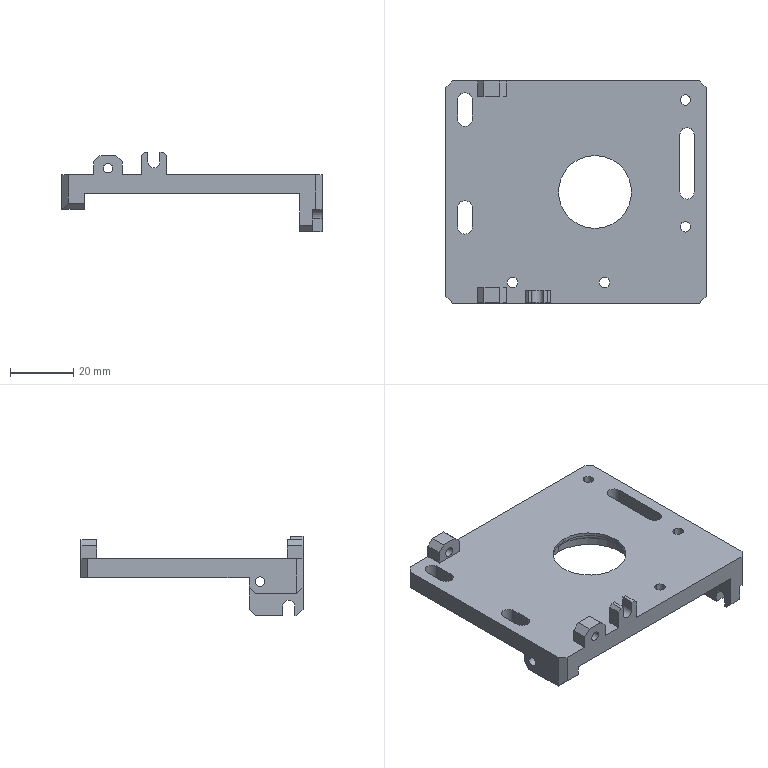NC program | NX | posted with a generic post | part box 82 x 70 x 25 mm
Lines 1 to 1408 of 8354:
N10 G17 G21 G94 G90
(FLOOR_WALL_COPY , TOOL : D20R0.8)
N12 T01 M6
N14 G54
N16 G17 G0 G90 X34.999 Y54. S7500 M3
N18 G43 Z30. H1
N20 Z3.
N22 G94 G1 Z0. F1350.
N24 Y51.
N26 Y-51.
N28 X26.051
N30 Y51.
N32 X17.102
N34 Y-51.
N36 X8.154
N38 Y51.
N40 X-0.795
N42 Y-51.
N44 X-9.743
N46 Y51.
N48 X-18.692
N50 Y-51.
N52 X-27.64
N54 Y51.
N56 Y54.
N58 Z3.
N60 G0 Z30.
N62 M5
(CAVITY_MILL_COPY_1_COPY , TOOL : D10)
N64 T10 M6
N66 G54
N68 G17 G0 G90 X-2.527 Y5.175 S9500 M3
N70 G43 Z30. H10
N72 Z-11.
N74 G94 G1 X-2.523 Y5.159 Z-11.001 F3000.
N76 X-2.259 Y4.595 Z-11.034
N78 X-1.87 Y4.108 Z-11.066
N80 X-1.378 Y3.725 Z-11.099
N82 X-0.811 Y3.467 Z-11.132
N84 X-0.199 Y3.347 Z-11.164
N86 X0.423 Y3.374 Z-11.197
N88 X1.023 Y3.544 Z-11.229
N90 X1.431 Y3.758 Z-11.254
N92 X1.903 Y4.141 Z-11.285
N94 X2.275 Y4.621 Z-11.317
N96 X2.528 Y5.174 Z-11.349
N98 X2.65 Y5.769 Z-11.381
N100 Y6.23 Z-11.405
N102 X2.517 Y6.862 Z-11.439
N104 X2.235 Y7.443 Z-11.473
N106 X1.821 Y7.939 Z-11.507
N108 X1.301 Y8.32 Z-11.541
N110 X0.982 Y8.464 Z-11.559
N112 X0.776 Y8.536 Z-11.57
N114 X0.459 Y8.62 Z-11.587
N116 X0.23 Y8.65 Z-11.6
N118 X-0.23 Z-11.624
N120 X-0.26 Y8.647 Z-11.625
N122 X-0.523 Y8.598 Z-11.639
N124 X-0.621 Y8.577 Z-11.645
N126 X-0.904 Y8.502 Z-11.66
N128 X-1.433 Y8.241 Z-11.691
N130 X-1.891 Y7.871 Z-11.722
N132 X-2.257 Y7.408 Z-11.753
N134 X-2.511 Y6.877 Z-11.783
N136 X-2.58 Y6.607 Z-11.798
N138 X-2.639 Y6.335 Z-11.813
N140 X-2.65 Y6.23 Z-11.818
N142 Y5.769 Z-11.842
N144 X-2.523 Y5.159 Z-11.875
N146 X-2.259 Y4.595 Z-11.908
N148 X-1.87 Y4.108 Z-11.94
N150 X-1.378 Y3.725 Z-11.973
N152 X-0.811 Y3.467 Z-12.006
N154 X-0.199 Y3.347 Z-12.038
N156 X0.423 Y3.374 Z-12.071
N158 X1.023 Y3.544 Z-12.104
N160 X1.431 Y3.758 Z-12.128
N162 X1.903 Y4.141 Z-12.16
N164 X2.275 Y4.621 Z-12.191
N166 X2.528 Y5.174 Z-12.223
N168 X2.65 Y5.769 Z-12.255
N170 Y6.23 Z-12.279
N172 X2.517 Y6.862 Z-12.313
N174 X2.235 Y7.443 Z-12.347
N176 X1.821 Y7.939 Z-12.381
N178 X1.301 Y8.32 Z-12.415
N180 X0.982 Y8.464 Z-12.433
N182 X0.776 Y8.536 Z-12.444
N184 X0.459 Y8.62 Z-12.462
N186 X0.23 Y8.65 Z-12.474
N188 X0. Z-12.486
N190 G3 X-2.65 Y6. R2.65
N192 X0. Y8.65 R-2.65
N194 G1 Y14.65
N196 G3 X-1.588 Y14.503 R8.65
N198 X-2.317 Y14.334 R8.65
N200 X-8.383 Y8.133 R8.65
N202 X-8.455 Y7.826 R8.65
N204 X2.836 Y14.172 R-8.65
N206 X2.057 Y14.402 R8.65
N208 X0. Y14.65 R8.65
N210 X-0.866 Y14.15 R1.
N212 G1 Z-11.486
N214 G0 Z30.
N216 X-0.828 Y8.522
N218 Z-11.486
N220 G1 X-0.904 Y8.502 Z-11.49
N222 X-1.427 Y8.245 Z-11.52
N224 X-1.881 Y7.881 Z-11.551
N226 X-2.245 Y7.427 Z-11.581
N228 X-2.502 Y6.904 Z-11.612
N230 X-2.577 Y6.621 Z-11.627
N232 X-2.639 Y6.335 Z-11.643
N234 X-2.65 Y6.23 Z-11.648
N236 Y5.769 Z-11.672
N238 X-2.523 Y5.159 Z-11.705
N240 X-2.259 Y4.595 Z-11.738
N242 X-1.87 Y4.108 Z-11.77
N244 X-1.378 Y3.725 Z-11.803
N246 X-0.811 Y3.467 Z-11.836
N248 X-0.199 Y3.347 Z-11.868
N250 X0.423 Y3.374 Z-11.901
N252 X1.023 Y3.544 Z-11.934
N254 X1.431 Y3.758 Z-11.958
N256 X1.903 Y4.141 Z-11.99
N258 X2.275 Y4.621 Z-12.021
N260 X2.528 Y5.174 Z-12.053
N262 X2.65 Y5.769 Z-12.085
N264 Y6. Z-12.097
N266 Y6.23 Z-12.109
N268 X2.639 Y6.334 Z-12.115
N270 X2.59 Y6.56 Z-12.127
N272 X2.577 Y6.621 Z-12.13
N274 X2.561 Y6.682 Z-12.133
N276 X2.502 Y6.904 Z-12.145
N278 X2.345 Y7.256 Z-12.166
N280 X2.092 Y7.642 Z-12.19
N282 X1.73 Y8.02 Z-12.217
N284 X1.301 Y8.32 Z-12.245
N286 X0.987 Y8.462 Z-12.263
N288 X0.782 Y8.534 Z-12.274
N290 X0.621 Y8.577 Z-12.283
N292 X0.56 Y8.59 Z-12.286
N294 X0.335 Y8.639 Z-12.298
N296 X0. Y8.66 Z-12.316
N298 X-0.335 Y8.639 Z-12.333
N300 X-0.56 Y8.59 Z-12.345
N302 X-0.621 Y8.577 Z-12.349
N304 X-0.904 Y8.502 Z-12.364
N306 X-1.427 Y8.245 Z-12.395
N308 X-1.881 Y7.881 Z-12.425
N310 X-2.245 Y7.427 Z-12.456
N312 X-2.502 Y6.904 Z-12.486
N314 X-2.577 Y6.621 Z-12.501
N316 X-2.639 Y6.335 Z-12.517
N318 X-2.65 Y6.23 Z-12.522
N320 Y5.769 Z-12.547
N322 X-2.523 Y5.159 Z-12.579
N324 X-2.259 Y4.595 Z-12.612
N326 X-1.87 Y4.108 Z-12.644
N328 X-1.378 Y3.725 Z-12.677
N330 X-0.811 Y3.467 Z-12.71
N332 X-0.199 Y3.347 Z-12.742
N334 X0.423 Y3.374 Z-12.775
N336 X1.023 Y3.544 Z-12.808
N338 X1.431 Y3.758 Z-12.832
N340 X1.903 Y4.141 Z-12.864
N342 X2.275 Y4.621 Z-12.896
N344 X2.528 Y5.174 Z-12.927
N346 X2.65 Y5.769 Z-12.959
N348 Y6. Z-12.971
N350 G3 X0. Y8.65 R2.65
N352 X2.65 Y6. R-2.65
N354 G1 X8.65
N356 G3 X8.455 Y7.827 R8.65
N358 X7.242 Y10.731 R8.65
N360 X2.873 Y14.159 R8.65
N362 X-8.455 Y7.827 R8.65
N364 X8.65 Y6. R-8.65
N366 X8.15 Y6.866 R1.
N368 G1 Z-11.971
N370 G0 Z30.
N372 X-2.526 Y5.173
N374 Z-11.971
N376 G1 X-2.523 Y5.159 Z-11.972
N378 X-2.259 Y4.595 Z-12.005
N380 X-1.87 Y4.108 Z-12.038
N382 X-1.378 Y3.725 Z-12.07
N384 X-0.811 Y3.467 Z-12.103
N386 X-0.199 Y3.347 Z-12.135
N388 X0.423 Y3.374 Z-12.168
N390 X1.023 Y3.544 Z-12.201
N392 X1.431 Y3.758 Z-12.225
N394 X1.903 Y4.141 Z-12.257
N396 X2.275 Y4.621 Z-12.289
N398 X2.528 Y5.174 Z-12.32
N400 X2.65 Y5.769 Z-12.352
N402 Y6.23 Z-12.376
N404 X2.517 Y6.862 Z-12.41
N406 X2.235 Y7.443 Z-12.444
N408 X1.821 Y7.939 Z-12.478
N410 X1.301 Y8.32 Z-12.512
N412 X0.881 Y8.51 Z-12.536
N414 X0.86 Y8.517 Z-12.537
N416 X0.598 Y8.582 Z-12.551
N418 X0.335 Y8.639 Z-12.565
N420 X0.23 Y8.65 Z-12.571
N422 X-0.23 Z-12.595
N424 X-0.335 Y8.639 Z-12.601
N426 X-0.56 Y8.59 Z-12.613
N428 X-0.621 Y8.577 Z-12.616
N430 X-0.904 Y8.502 Z-12.631
N432 X-1.424 Y8.247 Z-12.662
N434 X-1.876 Y7.886 Z-12.692
N436 X-2.239 Y7.436 Z-12.722
N438 X-2.496 Y6.918 Z-12.753
N440 X-2.617 Y6.474 Z-12.777
N442 X-2.65 Y6.23 Z-12.79
N444 Y5.769 Z-12.814
N446 X-2.523 Y5.159 Z-12.846
N448 X-2.259 Y4.595 Z-12.879
N450 X-1.87 Y4.108 Z-12.912
N452 X-1.378 Y3.725 Z-12.944
N454 X-0.811 Y3.467 Z-12.977
N456 X-0.199 Y3.347 Z-13.01
N458 X0.423 Y3.374 Z-13.042
N460 X1.023 Y3.544 Z-13.075
N462 X1.431 Y3.758 Z-13.099
N464 X1.903 Y4.141 Z-13.131
N466 X2.275 Y4.621 Z-13.163
N468 X2.528 Y5.174 Z-13.195
N470 X2.65 Y5.769 Z-13.227
N472 Y6.23 Z-13.251
N474 X2.517 Y6.862 Z-13.284
N476 X2.235 Y7.443 Z-13.318
N478 X1.821 Y7.939 Z-13.352
N480 X1.301 Y8.32 Z-13.386
N482 X0.881 Y8.51 Z-13.41
N484 X0.86 Y8.517 Z-13.411
N486 X0.598 Y8.582 Z-13.425
N488 X0.335 Y8.639 Z-13.44
N490 X0.23 Y8.65 Z-13.445
N492 X0. Z-13.457
N494 G3 X-2.65 Y6. R2.65
N496 X0. Y8.65 R-2.65
N498 G1 Y14.65
N500 G3 X-2.237 Y14.356 R8.65
N502 X-8.346 Y8.272 R8.65
N504 G1 X-8.361 Y8.217
N506 G3 X2.078 Y14.397 R-8.65
N508 X0. Y14.65 R8.65
N510 X-0.866 Y14.15 R1.
N512 G1 Z-12.457
N514 G0 X0.832 Y3.49
N516 G1 X1.023 Y3.544 Z-12.468
N518 X1.431 Y3.758 Z-12.492
N520 X1.903 Y4.141 Z-12.524
N522 X2.275 Y4.621 Z-12.555
N524 X2.528 Y5.174 Z-12.587
N526 X2.65 Y5.769 Z-12.619
N528 Y6.23 Z-12.643
N530 X2.639 Y6.335 Z-12.649
N532 X2.59 Y6.56 Z-12.661
N534 X2.577 Y6.621 Z-12.664
N536 X2.561 Y6.682 Z-12.667
N538 X2.502 Y6.904 Z-12.679
N540 X2.317 Y7.306 Z-12.703
N542 X2.069 Y7.672 Z-12.726
N544 X1.749 Y8.004 Z-12.75
N546 X1.301 Y8.32 Z-12.779
N548 X1.034 Y8.441 Z-12.794
N550 X0.831 Y8.521 Z-12.805
N552 X0.621 Y8.577 Z-12.817
N554 X0.335 Y8.639 Z-12.832
N556 X0. Y8.66 Z-12.85
N558 X-0.335 Y8.639 Z-12.867
N560 X-0.56 Y8.59 Z-12.879
N562 X-0.621 Y8.577 Z-12.883
N564 X-0.904 Y8.502 Z-12.898
N566 X-1.033 Y8.451 Z-12.905
N568 X-1.441 Y8.236 Z-12.929
N570 X-1.817 Y7.942 Z-12.955
N572 X-2.125 Y7.6 Z-12.979
N574 X-2.339 Y7.266 Z-12.999
N576 X-2.502 Y6.904 Z-13.02
N578 X-2.561 Y6.682 Z-13.032
N580 X-2.576 Y6.624 Z-13.035
N582 X-2.638 Y6.341 Z-13.051
N584 X-2.65 Y6.23 Z-13.056
N586 Y5.999 Z-13.069
N588 Y5.769 Z-13.081
N590 X-2.523 Y5.159 Z-13.113
N592 X-2.259 Y4.595 Z-13.146
N594 X-1.87 Y4.108 Z-13.179
N596 X-1.378 Y3.725 Z-13.211
N598 X-0.811 Y3.467 Z-13.244
N600 X-0.199 Y3.347 Z-13.277
N602 X0.423 Y3.374 Z-13.309
N604 X1.023 Y3.544 Z-13.342
N606 X1.431 Y3.758 Z-13.366
N608 X1.903 Y4.141 Z-13.398
N610 X2.275 Y4.621 Z-13.43
N612 X2.528 Y5.174 Z-13.462
N614 X2.65 Y5.769 Z-13.493
N616 Y6.23 Z-13.518
N618 X2.639 Y6.335 Z-13.523
N620 X2.59 Y6.56 Z-13.535
N622 X2.577 Y6.621 Z-13.538
N624 X2.561 Y6.682 Z-13.542
N626 X2.502 Y6.904 Z-13.554
N628 X2.317 Y7.306 Z-13.577
N630 X2.069 Y7.672 Z-13.6
N632 X1.749 Y8.004 Z-13.624
N634 X1.301 Y8.32 Z-13.653
N636 X1.034 Y8.441 Z-13.668
N638 X0.831 Y8.521 Z-13.68
N640 X0.621 Y8.577 Z-13.691
N642 X0.335 Y8.639 Z-13.707
N644 X0. Y8.66 Z-13.724
N646 X-0.335 Y8.639 Z-13.742
N648 X-0.56 Y8.59 Z-13.754
N650 X-0.621 Y8.577 Z-13.757
N652 X-0.904 Y8.502 Z-13.772
N654 X-1.033 Y8.451 Z-13.78
N656 X-1.441 Y8.236 Z-13.804
N658 X-1.817 Y7.942 Z-13.829
N660 X-2.125 Y7.6 Z-13.853
N662 X-2.339 Y7.266 Z-13.874
N664 X-2.502 Y6.904 Z-13.895
N666 X-2.561 Y6.682 Z-13.907
N668 X-2.576 Y6.624 Z-13.91
N670 X-2.638 Y6.341 Z-13.925
N672 X-2.65 Y6.23 Z-13.931
N674 Y6. Z-13.943
N676 G3 X0.001 Y3.35 R2.65
N678 X-2.65 Y6. R-2.65
N680 G1 X-8.65
N682 Y5.998
N684 G3 X8.455 Y7.828 R-8.65
N686 X6.23 Y12. R8.65
N688 X3.184 Y14.043 R8.65
N690 X-4.038 Y13.65 R8.65
N692 X-6.434 Y11.781 R8.65
N694 X-8.451 Y7.847 R8.65
N696 X-8.65 Y6. R8.65
N698 X-8.15 Y5.134 R1.
N700 G1 Z-12.943
N702 G0 X-2.525 Y5.168
N704 G1 X-2.523 Y5.159
N706 X-2.259 Y4.595 Z-12.976
N708 X-1.87 Y4.108 Z-13.009
N710 X-1.378 Y3.725 Z-13.041
N712 X-0.811 Y3.467 Z-13.074
N714 X-0.199 Y3.347 Z-13.107
N716 X0.423 Y3.374 Z-13.139
N718 X1.023 Y3.544 Z-13.172
N720 X1.431 Y3.758 Z-13.196
N722 X1.903 Y4.141 Z-13.228
N724 X2.275 Y4.621 Z-13.26
N726 X2.528 Y5.174 Z-13.292
N728 X2.65 Y5.769 Z-13.323
N730 Y6.23 Z-13.348
N732 X2.625 Y6.431 Z-13.358
N734 X2.524 Y6.828 Z-13.38
N736 X2.37 Y7.209 Z-13.401
N738 X2.022 Y7.728 Z-13.434
N740 X1.563 Y8.152 Z-13.467
N742 X1.168 Y8.39 Z-13.491
N744 X0.904 Y8.502 Z-13.506
N746 X0.621 Y8.577 Z-13.521
N748 X0.335 Y8.639 Z-13.537
N750 X0.23 Y8.65 Z-13.542
N752 X-0.23 Z-13.566
N754 X-0.335 Y8.639 Z-13.572
N756 X-0.621 Y8.577 Z-13.587
N758 X-0.904 Y8.502 Z-13.603
N760 X-1.331 Y8.303 Z-13.627
N762 X-1.716 Y8.033 Z-13.652
N764 X-2.041 Y7.706 Z-13.676
N766 X-2.169 Y7.539 Z-13.687
N768 X-2.402 Y7.142 Z-13.711
N770 X-2.502 Y6.904 Z-13.725
N772 X-2.577 Y6.621 Z-13.74
N774 X-2.59 Y6.56 Z-13.743
N776 X-2.639 Y6.335 Z-13.755
N778 X-2.65 Y6.23 Z-13.761
N780 Y5.769 Z-13.785
N782 X-2.523 Y5.159 Z-13.818
N784 X-2.259 Y4.595 Z-13.85
N786 X-1.87 Y4.108 Z-13.883
N788 X-1.378 Y3.725 Z-13.916
N790 X-0.811 Y3.467 Z-13.948
N792 X-0.199 Y3.347 Z-13.981
N794 X0.423 Y3.374 Z-14.014
N796 X1.023 Y3.544 Z-14.046
N798 X1.431 Y3.758 Z-14.07
N800 X1.903 Y4.141 Z-14.102
N802 X2.275 Y4.621 Z-14.134
N804 X2.528 Y5.174 Z-14.166
N806 X2.65 Y5.769 Z-14.198
N808 Y6.23 Z-14.222
N810 X2.625 Y6.431 Z-14.233
N812 X2.524 Y6.828 Z-14.254
N814 X2.37 Y7.209 Z-14.276
N816 X2.022 Y7.728 Z-14.308
N818 X1.563 Y8.152 Z-14.341
N820 X1.168 Y8.39 Z-14.365
N822 X0.904 Y8.502 Z-14.38
N824 X0.621 Y8.577 Z-14.396
N826 X0.335 Y8.639 Z-14.411
N828 X0.23 Y8.65 Z-14.416
N830 X0. Z-14.429
N832 G3 X-2.65 Y6. R2.65
N834 X0. Y8.65 R-2.65
N836 G1 Y14.65
N838 G3 X-6.131 Y12.102 R8.65
N840 X-7.462 Y10.376 R8.65
N842 X-8.455 Y7.826 R8.65
N844 X8.382 Y8.135 R-8.65
N846 X8.017 Y9.248 R8.65
N848 X4.458 Y13.413 R8.65
N850 X0. Y14.65 R8.65
N852 X-0.866 Y14.15 R1.
N854 G1 Z-13.429
N856 G0 X-2.526 Y5.17
N858 G1 X-2.523 Y5.159
N860 X-2.259 Y4.595 Z-13.462
N862 X-1.87 Y4.108 Z-13.494
N864 X-1.378 Y3.725 Z-13.527
N866 X-0.811 Y3.467 Z-13.56
N868 X-0.199 Y3.347 Z-13.592
N870 X0.423 Y3.374 Z-13.625
N872 X1.023 Y3.544 Z-13.658
N874 X1.431 Y3.758 Z-13.682
N876 X1.903 Y4.141 Z-13.714
N878 X2.275 Y4.621 Z-13.746
N880 X2.528 Y5.174 Z-13.777
N882 X2.65 Y5.769 Z-13.809
N884 Y6.23 Z-13.833
N886 X2.634 Y6.369 Z-13.841
N888 X2.583 Y6.594 Z-13.853
N890 X2.572 Y6.638 Z-13.855
N892 X2.561 Y6.682 Z-13.858
N894 X2.502 Y6.904 Z-13.87
N896 X2.305 Y7.328 Z-13.894
N898 X2.041 Y7.706 Z-13.918
N900 X1.699 Y8.047 Z-13.944
N902 X1.301 Y8.32 Z-13.969
N904 X0.881 Y8.51 Z-13.993
N906 X0.799 Y8.537 Z-13.998
N908 X0.514 Y8.6 Z-14.013
N910 X0.228 Y8.65 Z-14.028
N912 X-0.007 Z-14.04
N914 X-0.238 Y8.649 Z-14.053
N916 X-0.335 Y8.639 Z-14.058
N918 X-0.621 Y8.577 Z-14.073
N920 X-0.888 Y8.506 Z-14.088
N922 X-1.294 Y8.324 Z-14.111
N924 X-1.817 Y7.942 Z-14.145
N926 X-2.233 Y7.446 Z-14.179
N928 X-2.516 Y6.863 Z-14.213
N930 X-2.65 Y6.23 Z-14.247
N932 Y5.769 Z-14.271
N934 X-2.523 Y5.159 Z-14.303
N936 X-2.259 Y4.595 Z-14.336
N938 X-1.87 Y4.108 Z-14.369
N940 X-1.378 Y3.725 Z-14.401
N942 X-0.811 Y3.467 Z-14.434
N944 X-0.199 Y3.347 Z-14.467
N946 X0.423 Y3.374 Z-14.499
N948 X1.023 Y3.544 Z-14.532
N950 X1.431 Y3.758 Z-14.556
N952 X1.903 Y4.141 Z-14.588
N954 X2.275 Y4.621 Z-14.62
N956 X2.528 Y5.174 Z-14.652
N958 X2.65 Y5.769 Z-14.683
N960 Y6.23 Z-14.708
N962 X2.634 Y6.369 Z-14.715
N964 X2.583 Y6.594 Z-14.727
N966 X2.572 Y6.638 Z-14.729
N968 X2.561 Y6.682 Z-14.732
N970 X2.502 Y6.904 Z-14.744
N972 X2.305 Y7.328 Z-14.768
N974 X2.041 Y7.706 Z-14.793
N976 X1.699 Y8.047 Z-14.818
N978 X1.301 Y8.32 Z-14.843
N980 X0.881 Y8.51 Z-14.867
N982 X0.799 Y8.537 Z-14.872
N984 X0.514 Y8.6 Z-14.887
N986 X0.228 Y8.65 Z-14.902
N988 X0. Z-14.914
N990 X-0.007
N992 G3 X-2.65 Y5.993 R2.65
N994 X0. Y8.65 R-2.65
N996 G1 Y14.65
N998 X-0.023
N1000 G3 X-3.538 Y13.894 R8.65
N1002 X8.43 Y7.938 R-8.65
N1004 X7.092 Y10.953 R8.65
N1006 X1.875 Y14.444 R8.65
N1008 X1.478 Y14.523 R8.65
N1010 X0. Y14.65 R8.65
N1012 X-0.866 Y14.15 R1.
N1014 G1 Z-13.914
N1016 G0 X0.829 Y3.489
N1018 G1 X1.023 Y3.544 Z-13.925
N1020 X1.431 Y3.758 Z-13.949
N1022 X1.903 Y4.141 Z-13.981
N1024 X2.275 Y4.621 Z-14.013
N1026 X2.528 Y5.174 Z-14.045
N1028 X2.65 Y5.769 Z-14.076
N1030 Y6.23 Z-14.101
N1032 X2.525 Y6.838 Z-14.133
N1034 X2.262 Y7.4 Z-14.166
N1036 X1.876 Y7.886 Z-14.198
N1038 X1.387 Y8.27 Z-14.231
N1040 X0.975 Y8.475 Z-14.255
N1042 X0.904 Y8.502 Z-14.259
N1044 X0.621 Y8.577 Z-14.274
N1046 X0.335 Y8.639 Z-14.289
N1048 X0. Y8.66 Z-14.307
N1050 X-0.335 Y8.639 Z-14.325
N1052 X-0.621 Y8.577 Z-14.34
N1054 X-0.904 Y8.502 Z-14.355
N1056 X-1.083 Y8.43 Z-14.365
N1058 X-1.486 Y8.206 Z-14.39
N1060 X-1.842 Y7.919 Z-14.414
N1062 X-2.143 Y7.575 Z-14.438
N1064 X-2.382 Y7.185 Z-14.462
N1066 X-2.522 Y6.829 Z-14.482
N1068 X-2.577 Y6.621 Z-14.493
N1070 X-2.639 Y6.335 Z-14.508
N1072 X-2.65 Y6.23 Z-14.514
N1074 Y5.999 Z-14.526
N1076 Y5.769 Z-14.538
N1078 X-2.523 Y5.159 Z-14.571
N1080 X-2.259 Y4.595 Z-14.603
N1082 X-1.87 Y4.108 Z-14.636
N1084 X-1.378 Y3.725 Z-14.668
N1086 X-0.811 Y3.467 Z-14.701
N1088 X-0.199 Y3.347 Z-14.734
N1090 X0.423 Y3.374 Z-14.766
N1092 X1.023 Y3.544 Z-14.799
N1094 X1.431 Y3.758 Z-14.823
N1096 X1.903 Y4.141 Z-14.855
N1098 X2.275 Y4.621 Z-14.887
N1100 X2.528 Y5.174 Z-14.919
N1102 X2.65 Y5.769 Z-14.951
N1104 Y6.23 Z-14.975
N1106 X2.525 Y6.838 Z-15.007
N1108 X2.262 Y7.4 Z-15.04
N1110 X1.876 Y7.886 Z-15.072
N1112 X1.387 Y8.27 Z-15.105
N1114 X0.975 Y8.475 Z-15.129
N1116 X0.904 Y8.502 Z-15.133
N1118 X0.621 Y8.577 Z-15.148
N1120 X0.335 Y8.639 Z-15.164
N1122 X0. Y8.66 Z-15.181
N1124 X-0.335 Y8.639 Z-15.199
N1126 X-0.621 Y8.577 Z-15.214
N1128 X-0.904 Y8.502 Z-15.23
N1130 X-1.083 Y8.43 Z-15.24
N1132 X-1.486 Y8.206 Z-15.264
N1134 X-1.842 Y7.919 Z-15.288
N1136 X-2.143 Y7.575 Z-15.312
N1138 X-2.382 Y7.185 Z-15.336
N1140 X-2.522 Y6.829 Z-15.356
N1142 X-2.577 Y6.621 Z-15.367
N1144 X-2.639 Y6.335 Z-15.382
N1146 X-2.65 Y6.23 Z-15.388
N1148 Y6. Z-15.4
N1150 G3 X0.001 Y3.35 R2.65
N1152 X-2.65 Y6. R-2.65
N1154 G1 X-8.65
N1156 Y5.998
N1158 G3 X3.855 Y13.743 R-8.65
N1160 X-4.193 Y13.566 R8.65
N1162 X-8.049 Y9.167 R8.65
N1164 X-8.455 Y7.827 R8.65
N1166 X-8.65 Y6. R8.65
N1168 X-8.15 Y5.134 R1.
N1170 G1 Z-14.4
N1172 G0 X-5.547 Y10.905
N1174 G1 X-6.124 Y10.171 Z-14.449
N1176 X-6.636 Y9.298 Z-14.502
N1178 X-7.023 Y8.362 Z-14.555
N1180 X-7.28 Y7.383 Z-14.608
N1182 X-7.4 Y6.378 Z-14.661
N1184 Y5.608 Z-14.701
N1186 X-7.272 Y4.575 Z-14.756
N1188 X-7. Y3.571 Z-14.811
N1190 X-6.591 Y2.614 Z-14.865
N1192 X-6.052 Y1.724 Z-14.92
N1194 X-5.393 Y0.918 Z-14.974
N1196 X-4.628 Y0.213 Z-15.029
N1198 X-3.772 Y-0.378 Z-15.083
N1200 X-2.841 Y-0.844 Z-15.138
N1202 X-1.854 Y-1.174 Z-15.192
N1204 X-0.831 Y-1.363 Z-15.247
N1206 X0.209 Y-1.407 Z-15.301
N1208 X1.245 Y-1.305 Z-15.356
N1210 X2.256 Y-1.058 Z-15.41
N1212 X3.223 Y-0.673 Z-15.465
N1214 X3.897 Y-0.302 Z-15.505
N1216 X4.726 Y0.292 Z-15.559
N1218 X5.464 Y0.995 Z-15.612
N1220 X6.1 Y1.793 Z-15.666
N1222 X6.62 Y2.67 Z-15.719
N1224 X7.014 Y3.61 Z-15.773
N1226 X7.276 Y4.596 Z-15.826
N1228 X7.4 Y5.608 Z-15.879
N1230 Y6. Z-15.9
N1232 X1.4
N1234 G3 X0. Y7.4 R1.4
N1236 X1.4 Y6. R-1.4
N1238 G1 X7.4
N1240 G3 X0. Y13.4 R7.4
N1242 X7.4 Y6. R-7.4
N1244 X6.9 Y6.866 R1.
N1246 G1 Z-14.9
N1248 G0 X-5.547 Y10.905
N1250 G1 X-6.124 Y10.171 Z-14.949
N1252 X-6.636 Y9.298 Z-15.002
N1254 X-7.023 Y8.362 Z-15.055
N1256 X-7.28 Y7.383 Z-15.108
N1258 X-7.4 Y6.378 Z-15.161
N1260 Y5.608 Z-15.201
N1262 X-7.272 Y4.575 Z-15.256
N1264 X-7. Y3.571 Z-15.311
N1266 X-6.591 Y2.614 Z-15.365
N1268 X-6.052 Y1.724 Z-15.42
N1270 X-5.393 Y0.918 Z-15.474
N1272 X-4.628 Y0.213 Z-15.529
N1274 X-3.772 Y-0.378 Z-15.583
N1276 X-2.841 Y-0.844 Z-15.638
N1278 X-1.854 Y-1.174 Z-15.692
N1280 X-0.831 Y-1.363 Z-15.747
N1282 X0.209 Y-1.407 Z-15.801
N1284 X1.245 Y-1.305 Z-15.856
N1286 X2.256 Y-1.058 Z-15.91
N1288 X3.223 Y-0.673 Z-15.965
N1290 X3.897 Y-0.302 Z-16.005
N1292 X4.726 Y0.292 Z-16.059
N1294 X5.464 Y0.995 Z-16.112
N1296 X6.1 Y1.793 Z-16.166
N1298 X6.62 Y2.67 Z-16.219
N1300 X7.014 Y3.61 Z-16.273
N1302 X7.276 Y4.596 Z-16.326
N1304 X7.4 Y5.608 Z-16.379
N1306 Y6. Z-16.4
N1308 X1.4
N1310 G3 X0. Y7.4 R1.4
N1312 X1.4 Y6. R-1.4
N1314 G1 X7.4
N1316 G3 X0. Y13.4 R7.4
N1318 X7.4 Y6. R-7.4
N1320 X6.9 Y6.866 R1.
N1322 G1 Z-15.4
N1324 G0 X-5.547 Y10.905
N1326 G1 X-6.124 Y10.171 Z-15.449
N1328 X-6.636 Y9.298 Z-15.502
N1330 X-7.023 Y8.362 Z-15.555
N1332 X-7.28 Y7.383 Z-15.608
N1334 X-7.4 Y6.378 Z-15.661
N1336 Y5.608 Z-15.701
N1338 X-7.272 Y4.575 Z-15.756
N1340 X-7. Y3.571 Z-15.811
N1342 X-6.591 Y2.614 Z-15.865
N1344 X-6.052 Y1.724 Z-15.92
N1346 X-5.393 Y0.918 Z-15.974
N1348 X-4.628 Y0.213 Z-16.029
N1350 X-3.772 Y-0.378 Z-16.083
N1352 X-2.841 Y-0.844 Z-16.138
N1354 X-1.854 Y-1.174 Z-16.192
N1356 X-0.831 Y-1.363 Z-16.247
N1358 X0.209 Y-1.407 Z-16.301
N1360 X1.245 Y-1.305 Z-16.356
N1362 X2.256 Y-1.058 Z-16.41
N1364 X3.223 Y-0.673 Z-16.465
N1366 X3.897 Y-0.302 Z-16.505
N1368 X4.726 Y0.292 Z-16.559
N1370 X5.464 Y0.995 Z-16.612
N1372 X6.1 Y1.793 Z-16.666
N1374 X6.62 Y2.67 Z-16.719
N1376 X7.014 Y3.61 Z-16.773
N1378 X7.276 Y4.596 Z-16.826
N1380 X7.4 Y5.608 Z-16.879
N1382 Y6. Z-16.9
N1384 X1.4
N1386 G3 X0. Y7.4 R1.4
N1388 X1.4 Y6. R-1.4
N1390 G1 X7.4
N1392 G3 X0. Y13.4 R7.4
N1394 X7.4 Y6. R-7.4
N1396 X6.9 Y6.866 R1.
N1398 G1 Z-15.9
N1400 G0 X-5.131 Y2.173
N1402 G1 X-5.058 Y2.063 Z-15.907
N1404 X-4.407 Y1.345 Z-15.958
N1406 X-3.655 Y0.734 Z-16.008
N1408 X-2.82 Y0.244 Z-16.059
N1410 X-1.92 Y-0.116 Z-16.11
N1412 X-0.976 Y-0.335 Z-16.161
N1414 X-0.01 Y-0.41 Z-16.212
N1416 X0.956 Y-0.338 Z-16.262
N1418 X1.901 Y-0.122 Z-16.313
N1420 X2.802 Y0.235 Z-16.364
N1422 X3.427 Y0.583 Z-16.401
N1424 X4.129 Y1.097 Z-16.447
N1426 X4.754 Y1.701 Z-16.493
N1428 X5.293 Y2.384 Z-16.538
N1430 X5.734 Y3.134 Z-16.584
N1432 X6.069 Y3.936 Z-16.629
N1434 X6.292 Y4.777 Z-16.675
N1436 X6.4 Y5.64 Z-16.721
N1438 Y6.356 Z-16.758
N1440 X6.281 Y7.279 Z-16.807
N1442 X6.03 Y8.175 Z-16.856
N1444 X5.651 Y9.025 Z-16.904
N1446 X5.154 Y9.811 Z-16.953
N1448 X4.548 Y10.517 Z-17.002
N1450 X3.846 Y11.128 Z-17.051
N1452 X3.063 Y11.631 Z-17.099
N1454 X2.416 Y11.937 Z-17.137
N1456 X1.748 Y12.167 Z-17.174
N1458 X1.06 Y12.322 Z-17.211
N1460 X0.358 Y12.4 Z-17.248
N1462 X0. Z-17.267
N1464 Y6.4
N1466 G3 X-0.4 Y6. R0.4
N1468 X0. Y6.4 R-0.4
N1470 G1 Y12.4
N1472 G3 X-6.4 Y6. R6.4
N1474 X0. Y12.4 R-6.4
N1476 X-0.866 Y11.9 R1.
N1478 G1 Z-16.267
N1480 G0 X-5.131 Y2.173
N1482 G1 X-5.058 Y2.063 Z-16.274
N1484 X-4.407 Y1.345 Z-16.324
N1486 X-3.655 Y0.734 Z-16.375
N1488 X-2.82 Y0.244 Z-16.426
N1490 X-1.92 Y-0.116 Z-16.477
N1492 X-0.976 Y-0.335 Z-16.527
N1494 X-0.01 Y-0.41 Z-16.578
N1496 X0.956 Y-0.338 Z-16.629
N1498 X1.901 Y-0.122 Z-16.68
N1500 X2.802 Y0.235 Z-16.731
N1502 X3.427 Y0.583 Z-16.768
N1504 X4.129 Y1.097 Z-16.814
N1506 X4.754 Y1.701 Z-16.859
N1508 X5.293 Y2.384 Z-16.905
N1510 X5.734 Y3.134 Z-16.95
N1512 X6.069 Y3.936 Z-16.996
N1514 X6.292 Y4.777 Z-17.042
N1516 X6.4 Y5.64 Z-17.087
N1518 Y6.356 Z-17.125
N1520 X6.281 Y7.279 Z-17.173
N1522 X6.03 Y8.175 Z-17.222
N1524 X5.651 Y9.025 Z-17.271
N1526 X5.154 Y9.811 Z-17.32
N1528 X4.548 Y10.517 Z-17.369
N1530 X3.846 Y11.128 Z-17.417
N1532 X3.063 Y11.631 Z-17.466
N1534 X2.416 Y11.937 Z-17.504
N1536 X1.748 Y12.167 Z-17.541
N1538 X1.06 Y12.322 Z-17.578
N1540 X0.358 Y12.4 Z-17.615
N1542 X0. Z-17.633
N1544 Y6.4
N1546 G3 X-0.4 Y6. R0.4
N1548 X0. Y6.4 R-0.4
N1550 G1 Y12.4
N1552 G3 X-6.4 Y6. R6.4
N1554 X0. Y12.4 R-6.4
N1556 X-0.866 Y11.9 R1.
N1558 G1 Z-16.633
N1560 G0 X-5.131 Y2.173
N1562 G1 X-5.058 Y2.063 Z-16.64
N1564 X-4.407 Y1.345 Z-16.691
N1566 X-3.655 Y0.734 Z-16.742
N1568 X-2.82 Y0.244 Z-16.793
N1570 X-1.92 Y-0.116 Z-16.843
N1572 X-0.976 Y-0.335 Z-16.894
N1574 X-0.01 Y-0.41 Z-16.945
N1576 X0.956 Y-0.338 Z-16.996
N1578 X1.901 Y-0.122 Z-17.046
N1580 X2.802 Y0.235 Z-17.097
N1582 X3.427 Y0.583 Z-17.135
N1584 X4.129 Y1.097 Z-17.18
N1586 X4.754 Y1.701 Z-17.226
N1588 X5.293 Y2.384 Z-17.272
N1590 X5.734 Y3.134 Z-17.317
N1592 X6.069 Y3.936 Z-17.363
N1594 X6.292 Y4.777 Z-17.408
N1596 X6.4 Y5.64 Z-17.454
N1598 Y6.356 Z-17.491
N1600 X6.281 Y7.279 Z-17.54
N1602 X6.03 Y8.175 Z-17.589
N1604 X5.651 Y9.025 Z-17.638
N1606 X5.154 Y9.811 Z-17.686
N1608 X4.548 Y10.517 Z-17.735
N1610 X3.846 Y11.128 Z-17.784
N1612 X3.063 Y11.631 Z-17.833
N1614 X2.416 Y11.937 Z-17.87
N1616 X1.748 Y12.167 Z-17.907
N1618 X1.06 Y12.322 Z-17.944
N1620 X0.358 Y12.4 Z-17.981
N1622 X0. Z-18.
N1624 Y6.4
N1626 G3 X-0.4 Y6. R0.4
N1628 X0. Y6.4 R-0.4
N1630 G1 Y12.4
N1632 G3 X-6.4 Y6. R6.4
N1634 X0. Y12.4 R-6.4
N1636 X-0.866 Y11.9 R1.
N1638 G1 Z-17.
N1640 G0 X-6.208 Y4.458
N1642 G1 X-6.002 Y3.749 Z-17.039
N1644 X-5.594 Y2.87 Z-17.089
N1646 X-5.058 Y2.063 Z-17.14
N1648 X-4.407 Y1.345 Z-17.191
N1650 X-3.655 Y0.734 Z-17.242
N1652 X-2.819 Y0.243 Z-17.293
N1654 X-1.919 Y-0.116 Z-17.343
N1656 X-0.976 Y-0.335 Z-17.394
N1658 X-0.01 Y-0.41 Z-17.445
N1660 X0.957 Y-0.338 Z-17.496
N1662 X1.901 Y-0.122 Z-17.547
N1664 X2.802 Y0.235 Z-17.597
N1666 X3.428 Y0.583 Z-17.635
N1668 X4.129 Y1.097 Z-17.68
N1670 X4.755 Y1.701 Z-17.726
N1672 X5.293 Y2.384 Z-17.772
N1674 X5.734 Y3.134 Z-17.817
N1676 X6.069 Y3.937 Z-17.863
N1678 X6.292 Y4.777 Z-17.908
N1680 X6.4 Y5.64 Z-17.954
N1682 Y6.356 Z-17.991
N1684 X6.281 Y7.279 Z-18.04
N1686 X6.03 Y8.175 Z-18.089
N1688 X5.651 Y9.026 Z-18.138
N1690 X5.153 Y9.812 Z-18.186
N1692 X4.547 Y10.518 Z-18.235
N1694 X3.845 Y11.129 Z-18.284
N1696 X3.061 Y11.632 Z-18.333
N1698 X2.414 Y11.938 Z-18.37
N1700 X1.747 Y12.167 Z-18.407
N1702 X1.059 Y12.322 Z-18.444
N1704 X0.358 Y12.4 Z-18.481
N1706 X0. Z-18.5
N1708 Y6.4
N1710 G3 X-0.4 Y6. R0.4
N1712 X0. Y6.4 R-0.4
N1714 G1 Y12.4
N1716 G3 X-6.4 Y6. R6.4
N1718 X0. Y12.4 R-6.4
N1720 X-0.866 Y11.9 R1.
N1722 G1 Z-17.5
N1724 G0 Z30.
N1726 M5
(FLOOR_WALL_1_COPY , TOOL : D4)
N1728 T04 M6
N1730 G54
N1732 G17 G0 G90 X-36. Y-34.001 S9500 M3
N1734 G43 Z30. H4
N1736 Z-6.5
N1738 G94 G1 Z-7. F1350.
N1740 X-35.
N1742 X-18.
N1744 Y-35.801
N1746 X-35.
N1748 Y-37.6
N1750 X-18.
N1752 Y-39.4
N1754 X-35.
N1756 X-36.
N1758 Z-6.5
N1760 G0 Z30.
N1762 X37.244 Y-40.999
N1764 Z-11.5
N1766 G1 Z-12.
N1768 X35.829
N1770 X-15.8
N1772 Y-39.038
N1774 X37.
N1776 Y-37.077
N1778 X-15.8
N1780 Y-35.116
N1782 X37.
N1784 Y-33.155
N1786 X-15.8
N1788 Y-32.
N1790 G3 X-16. Y-31.8 R0.2
N1792 G1 X-37.
N1794 Y-31.194
N1796 X37.
N1798 Y-29.233
N1800 X-37.
N1802 Y-27.272
N1804 X37.
N1806 Y-25.311
N1808 X-37.
N1810 Y-23.35
N1812 X37.
N1814 Y-21.389
N1816 X-37.
N1818 Y-19.429
N1820 X37.
N1822 Y-17.468
N1824 X-37.
N1826 Y-15.507
N1828 X37.
N1830 Y-13.546
N1832 X-37.
N1834 Y-11.585
N1836 X37.
N1838 Y-9.624
N1840 X-37.
N1842 Y-7.663
N1844 X37.
N1846 Y-5.702
N1848 X-37.
N1850 Y-3.741
N1852 X37.
N1854 Y-1.78
N1856 X-37.
N1858 Y0.181
N1860 X37.
N1862 Y2.142
N1864 X-37.
N1866 Y4.103
N1868 X37.
N1870 Y6.064
N1872 X-37.
N1874 Y8.025
N1876 X37.
N1878 Y9.986
N1880 X-37.
N1882 Y11.947
N1884 X37.
N1886 Y13.908
N1888 X-37.
N1890 Y15.869
N1892 X37.
N1894 Y17.83
N1896 X-37.
N1898 Y19.79
N1900 X37.
N1902 Y21.751
N1904 X-37.
N1906 Y23.712
N1908 X37.
N1910 Y25.673
N1912 X-37.
N1914 Y27.634
N1916 X37.
N1918 Y29.595
N1920 X-37.
N1922 Y31.556
N1924 X37.
N1926 Y33.517
N1928 X-15.8
N1930 Y35.478
N1932 X37.
N1934 Y37.439
N1936 X-15.8
N1938 Y39.4
N1940 X37.
N1942 Y39.828
N1944 X35.467 Y41.361
N1946 X-15.8
N1948 Y44.
N1950 Z-11.5
N1952 G0 Z30.
N1954 X-16.
N1956 Z-11.5
N1958 G1 Z-12.
N1960 Y43.
N1962 Y32.
N1964 X-37.
N1966 X-38.
N1968 Z-11.5
N1970 G0 Z30.
N1972 Y-32.
N1974 Z-11.5
N1976 G1 Z-12.
N1978 X-37.
N1980 X-16.
N1982 Y-43.
N1984 Y-44.
N1986 Z-11.5
N1988 G0 Z30.
(FLOOR_WALL_1_COPY_COPY_1 , TOOL : D4)
N1990 X0. Y16.75
N1992 Z-15.
N1994 G1 Z-15.5
N1996 Y17.75
N1998 G3 X-11.75 Y6. R11.75
N2000 X0. Y17.75 R-11.75
N2002 G1 Y16.75
N2004 Z-15.
N2006 G0 Z30.
N2008 Y15.5
N2010 Z-16.5
N2012 G1 Z-17.
N2014 Y16.5
N2016 G3 X-10.5 Y6. R10.5
N2018 X0. Y16.5 R-10.5
N2020 G1 Y15.5
N2022 Z-16.5
N2024 G0 Z30.
(ZLEVEL_PROFILE_COPY_COPY , TOOL : D4)
N2026 X0.244 Y15.417
N2028 Z-14.
N2030 G1 Z-15.5 F1000.
N2032 G3 X0. Y15.5 R0.4
N2034 X-9.5 Y6. R9.5 F1500.
N2036 X0. Y15.5 R-9.5
N2038 G1 X-0.243 Y15.49 Z-15.508
N2040 X-0.486 Y15.48 Z-15.516
N2042 X-0.729 Y15.469 Z-15.524
N2044 X-0.971 Y15.444 Z-15.533
N2046 X-1.212 Y15.414 Z-15.541
N2048 X-1.453 Y15.384 Z-15.549
N2050 X-1.693 Y15.343 Z-15.557
N2052 X-1.931 Y15.292 Z-15.565
N2054 X-2.169 Y15.243 Z-15.573
N2056 X-2.406 Y15.187 Z-15.582
N2058 X-2.639 Y15.117 Z-15.59
N2060 X-2.872 Y15.048 Z-15.598
N2062 X-3.104 Y14.977 Z-15.606
N2064 X-3.331 Y14.889 Z-15.614
N2066 X-3.558 Y14.801 Z-15.622
N2068 X-3.784 Y14.712 Z-15.63
N2070 X-4.004 Y14.608 Z-15.639
N2072 X-4.222 Y14.5 Z-15.647
N2074 X-4.441 Y14.394 Z-15.655
N2076 X-4.653 Y14.276 Z-15.663
N2078 X-4.862 Y14.152 Z-15.671
N2080 X-5.071 Y14.027 Z-15.679
N2082 X-5.276 Y13.896 Z-15.688
N2084 X-5.473 Y13.754 Z-15.696
N2086 X-5.672 Y13.613 Z-15.704
N2088 X-5.868 Y13.469 Z-15.712
N2090 X-6.053 Y13.312 Z-15.72
N2092 X-6.239 Y13.155 Z-15.728
N2094 X-6.424 Y12.997 Z-15.736
N2096 X-6.597 Y12.826 Z-15.745
N2098 X-6.769 Y12.654 Z-15.753
N2100 X-6.94 Y12.482 Z-15.761
N2102 X-7.101 Y12.3 Z-15.769
N2104 X-7.259 Y12.114 Z-15.777
N2106 X-7.416 Y11.929 Z-15.785
N2108 X-7.565 Y11.737 Z-15.793
N2110 X-7.707 Y11.539 Z-15.802
N2112 X-7.849 Y11.342 Z-15.81
N2114 X-7.985 Y11.141 Z-15.818
N2116 X-8.11 Y10.932 Z-15.826
N2118 X-8.234 Y10.723 Z-15.834
N2120 X-8.358 Y10.513 Z-15.842
N2122 X-8.465 Y10.295 Z-15.851
N2124 X-8.572 Y10.077 Z-15.859
N2126 X-8.679 Y9.858 Z-15.867
N2128 X-8.77 Y9.633 Z-15.875
N2130 X-8.859 Y9.406 Z-15.883
N2132 X-8.948 Y9.18 Z-15.891
N2134 X-9.025 Y8.95 Z-15.899
N2136 X-9.094 Y8.716 Z-15.908
N2138 X-9.164 Y8.483 Z-15.916
N2140 X-9.227 Y8.248 Z-15.924
N2142 X-9.276 Y8.01 Z-15.932
N2144 X-9.326 Y7.772 Z-15.94
N2146 X-9.374 Y7.534 Z-15.948
N2148 X-9.404 Y7.293 Z-15.957
N2150 X-9.434 Y7.051 Z-15.965
N2152 X-9.464 Y6.81 Z-15.973
N2154 X-9.477 Y6.567 Z-15.981
N2156 X-9.485 Y6.324 Z-15.989
N2158 X-9.496 Y6.081 Z-15.997
N2160 X-9.493 Y5.838 Z-16.005
N2162 X-9.483 Y5.595 Z-16.014
N2164 X-9.473 Y5.352 Z-16.022
N2166 X-9.454 Y5.11 Z-16.03
N2168 X-9.423 Y4.868 Z-16.038
N2170 X-9.394 Y4.627 Z-16.046
N2172 X-9.36 Y4.386 Z-16.054
N2174 X-9.31 Y4.148 Z-16.063
N2176 X-9.26 Y3.91 Z-16.071
N2178 X-9.209 Y3.672 Z-16.079
N2180 X-9.141 Y3.439 Z-16.087
N2182 X-9.071 Y3.206 Z-16.095
N2184 X-9.001 Y2.973 Z-16.103
N2186 X-8.917 Y2.745 Z-16.111
N2188 X-8.829 Y2.518 Z-16.12
N2190 X-8.742 Y2.291 Z-16.128
N2192 X-8.643 Y2.069 Z-16.136
N2194 X-8.536 Y1.851 Z-16.144
N2196 X-8.43 Y1.632 Z-16.152
N2198 X-8.318 Y1.416 Z-16.16
N2200 X-8.193 Y1.207 Z-16.168
N2202 X-8.068 Y0.999 Z-16.177
N2204 X-7.942 Y0.791 Z-16.185
N2206 X-7.802 Y0.592 Z-16.193
N2208 X-7.661 Y0.394 Z-16.201
N2210 X-7.519 Y0.196 Z-16.209
N2212 X-7.364 Y0.009 Z-16.217
N2214 X-7.207 Y-0.177 Z-16.226
N2216 X-7.05 Y-0.362 Z-16.234
N2218 X-6.884 Y-0.54 Z-16.242
N2220 X-6.711 Y-0.711 Z-16.25
N2222 X-6.54 Y-0.884 Z-16.258
N2224 X-6.362 Y-1.05 Z-16.266
N2226 X-6.177 Y-1.207 Z-16.274
N2228 X-5.991 Y-1.364 Z-16.283
N2230 X-5.804 Y-1.519 Z-16.291
N2232 X-5.606 Y-1.661 Z-16.299
N2234 X-5.408 Y-1.802 Z-16.307
N2236 X-5.209 Y-1.942 Z-16.315
N2238 X-5.001 Y-2.068 Z-16.323
N2240 X-4.793 Y-2.193 Z-16.332
N2242 X-4.584 Y-2.318 Z-16.34
N2244 X-4.368 Y-2.43 Z-16.348
N2246 X-4.149 Y-2.536 Z-16.356
N2248 X-3.931 Y-2.643 Z-16.364
N2250 X-3.709 Y-2.742 Z-16.372
N2252 X-3.482 Y-2.829 Z-16.38
N2254 X-3.255 Y-2.917 Z-16.389
N2256 X-3.027 Y-3.001 Z-16.397
N2258 X-2.794 Y-3.071 Z-16.405
N2260 X-2.561 Y-3.141 Z-16.413
N2262 X-2.328 Y-3.209 Z-16.421
N2264 X-2.09 Y-3.26 Z-16.429
N2266 X-1.852 Y-3.31 Z-16.438
N2268 X-1.614 Y-3.36 Z-16.446
N2270 X-1.373 Y-3.394 Z-16.454
N2272 X-1.132 Y-3.423 Z-16.462
N2274 X-0.89 Y-3.454 Z-16.47
N2276 X-0.648 Y-3.473 Z-16.478
N2278 X-0.405 Y-3.483 Z-16.486
N2280 X-0.162 Y-3.493 Z-16.495
N2282 X0.081 Y-3.496 Z-16.503
N2284 X0.324 Y-3.485 Z-16.511
N2286 X0.567 Y-3.477 Z-16.519
N2288 X0.81 Y-3.464 Z-16.527
N2290 X1.051 Y-3.434 Z-16.535
N2292 X1.293 Y-3.404 Z-16.543
N2294 X1.534 Y-3.374 Z-16.552
N2296 X1.772 Y-3.326 Z-16.56
N2298 X2.01 Y-3.276 Z-16.568
N2300 X2.248 Y-3.227 Z-16.576
N2302 X2.483 Y-3.164 Z-16.584
N2304 X2.716 Y-3.094 Z-16.592
N2306 X2.95 Y-3.025 Z-16.601
N2308 X3.18 Y-2.948 Z-16.609
N2310 X3.406 Y-2.859 Z-16.617
N2312 X3.633 Y-2.77 Z-16.625
N2314 X3.858 Y-2.679 Z-16.633
N2316 X4.077 Y-2.572 Z-16.641
N2318 X4.295 Y-2.465 Z-16.649
N2320 X4.513 Y-2.358 Z-16.658
N2322 X4.723 Y-2.234 Z-16.666
N2324 X4.932 Y-2.11 Z-16.674
N2326 X5.141 Y-1.985 Z-16.682
N2328 X5.342 Y-1.849 Z-16.69
N2330 X5.539 Y-1.707 Z-16.698
N2332 X5.737 Y-1.565 Z-16.707
N2334 X5.929 Y-1.416 Z-16.715
N2336 X6.114 Y-1.259 Z-16.723
N2338 X6.3 Y-1.101 Z-16.731
N2340 X6.482 Y-0.94 Z-16.739
N2342 X6.654 Y-0.769 Z-16.747
N2344 X6.826 Y-0.597 Z-16.755
N2346 X6.997 Y-0.424 Z-16.764
N2348 X7.155 Y-0.239 Z-16.772
N2350 X7.312 Y-0.053 Z-16.78
N2352 X7.469 Y0.132 Z-16.788
N2354 X7.613 Y0.328 Z-16.796
N2356 X7.754 Y0.527 Z-16.804
N2358 X7.896 Y0.724 Z-16.813
N2360 X8.027 Y0.929 Z-16.821
N2362 X8.152 Y1.138 Z-16.829
N2364 X8.276 Y1.347 Z-16.837
N2366 X8.394 Y1.559 Z-16.845
N2368 X8.5 Y1.778 Z-16.853
N2370 X8.608 Y1.996 Z-16.861
N2372 X8.712 Y2.216 Z-16.87
N2374 X8.801 Y2.442 Z-16.878
N2376 X8.889 Y2.669 Z-16.886
N2378 X8.977 Y2.896 Z-16.894
N2380 X9.048 Y3.128 Z-16.902
N2382 X9.117 Y3.361 Z-16.91
N2384 X9.187 Y3.594 Z-16.918
N2386 X9.243 Y3.831 Z-16.927
N2388 X9.292 Y4.069 Z-16.935
N2390 X9.343 Y4.307 Z-16.943
N2392 X9.384 Y4.547 Z-16.951
N2394 X9.414 Y4.788 Z-16.959
N2396 X9.444 Y5.029 Z-16.967
N2398 X9.469 Y5.271 Z-16.976
N2400 X9.48 Y5.514 Z-16.984
N2402 X9.49 Y5.757 Z-16.992
N2404 X9.5 Y6. Z-17.
N2406 Y6.015
N2408 G3 X0. Y15.5 R9.5
N2410 G1 X-0.243 Y15.49 Z-17.005
N2412 X-0.486 Y15.48 Z-17.011
N2414 X-0.729 Y15.469 Z-17.016
N2416 X-0.971 Y15.444 Z-17.022
N2418 X-1.212 Y15.414 Z-17.027
N2420 X-1.453 Y15.384 Z-17.033
N2422 X-1.693 Y15.343 Z-17.038
N2424 X-1.931 Y15.292 Z-17.043
N2426 X-2.169 Y15.243 Z-17.049
N2428 X-2.406 Y15.187 Z-17.054
N2430 X-2.639 Y15.117 Z-17.06
N2432 X-2.872 Y15.048 Z-17.065
N2434 X-3.104 Y14.977 Z-17.071
N2436 X-3.331 Y14.889 Z-17.076
N2438 X-3.558 Y14.801 Z-17.082
N2440 X-3.784 Y14.712 Z-17.087
N2442 X-4.004 Y14.608 Z-17.092
N2444 X-4.222 Y14.5 Z-17.098
N2446 X-4.441 Y14.394 Z-17.103
N2448 X-4.653 Y14.276 Z-17.109
N2450 X-4.862 Y14.152 Z-17.114
N2452 X-5.071 Y14.027 Z-17.12
N2454 X-5.276 Y13.896 Z-17.125
N2456 X-5.473 Y13.754 Z-17.13
N2458 X-5.672 Y13.613 Z-17.136
N2460 X-5.868 Y13.469 Z-17.141
N2462 X-6.053 Y13.312 Z-17.147
N2464 X-6.239 Y13.155 Z-17.152
N2466 X-6.424 Y12.997 Z-17.158
N2468 X-6.597 Y12.826 Z-17.163
N2470 X-6.769 Y12.654 Z-17.168
N2472 X-6.94 Y12.482 Z-17.174
N2474 X-7.101 Y12.3 Z-17.179
N2476 X-7.259 Y12.114 Z-17.185
N2478 X-7.416 Y11.929 Z-17.19
N2480 X-7.565 Y11.737 Z-17.196
N2482 X-7.707 Y11.539 Z-17.201
N2484 X-7.849 Y11.342 Z-17.207
N2486 X-7.985 Y11.141 Z-17.212
N2488 X-8.11 Y10.932 Z-17.217
N2490 X-8.234 Y10.723 Z-17.223
N2492 X-8.358 Y10.513 Z-17.228
N2494 X-8.465 Y10.295 Z-17.234
N2496 X-8.572 Y10.077 Z-17.239
N2498 X-8.679 Y9.858 Z-17.245
N2500 X-8.77 Y9.633 Z-17.25
N2502 X-8.859 Y9.406 Z-17.255
N2504 X-8.948 Y9.18 Z-17.261
N2506 X-9.025 Y8.95 Z-17.266
N2508 X-9.094 Y8.716 Z-17.272
N2510 X-9.164 Y8.483 Z-17.277
N2512 X-9.227 Y8.248 Z-17.283
N2514 X-9.276 Y8.01 Z-17.288
N2516 X-9.326 Y7.772 Z-17.293
N2518 X-9.374 Y7.534 Z-17.299
N2520 X-9.404 Y7.293 Z-17.304
N2522 X-9.434 Y7.051 Z-17.31
N2524 X-9.464 Y6.81 Z-17.315
N2526 X-9.477 Y6.567 Z-17.321
N2528 X-9.485 Y6.324 Z-17.326
N2530 X-9.496 Y6.081 Z-17.332
N2532 X-9.493 Y5.838 Z-17.337
N2534 X-9.483 Y5.595 Z-17.342
N2536 X-9.473 Y5.352 Z-17.348
N2538 X-9.454 Y5.11 Z-17.353
N2540 X-9.423 Y4.868 Z-17.359
N2542 X-9.394 Y4.627 Z-17.364
N2544 X-9.36 Y4.386 Z-17.37
N2546 X-9.31 Y4.148 Z-17.375
N2548 X-9.26 Y3.91 Z-17.38
N2550 X-9.209 Y3.672 Z-17.386
N2552 X-9.141 Y3.439 Z-17.391
N2554 X-9.071 Y3.206 Z-17.397
N2556 X-9.001 Y2.973 Z-17.402
N2558 X-8.917 Y2.745 Z-17.408
N2560 X-8.829 Y2.518 Z-17.413
N2562 X-8.742 Y2.291 Z-17.418
N2564 X-8.643 Y2.069 Z-17.424
N2566 X-8.536 Y1.851 Z-17.429
N2568 X-8.43 Y1.632 Z-17.435
N2570 X-8.318 Y1.416 Z-17.44
N2572 X-8.193 Y1.207 Z-17.446
N2574 X-8.068 Y0.999 Z-17.451
N2576 X-7.942 Y0.791 Z-17.457
N2578 X-7.802 Y0.592 Z-17.462
N2580 X-7.661 Y0.394 Z-17.467
N2582 X-7.519 Y0.196 Z-17.473
N2584 X-7.364 Y0.009 Z-17.478
N2586 X-7.207 Y-0.177 Z-17.484
N2588 X-7.05 Y-0.362 Z-17.489
N2590 X-6.884 Y-0.54 Z-17.495
N2592 X-6.711 Y-0.711 Z-17.5
N2594 X-6.54 Y-0.884 Z-17.505
N2596 X-6.362 Y-1.05 Z-17.511
N2598 X-6.177 Y-1.207 Z-17.516
N2600 X-5.991 Y-1.364 Z-17.522
N2602 X-5.804 Y-1.519 Z-17.527
N2604 X-5.606 Y-1.661 Z-17.533
N2606 X-5.408 Y-1.802 Z-17.538
N2608 X-5.209 Y-1.942 Z-17.543
N2610 X-5.001 Y-2.068 Z-17.549
N2612 X-4.793 Y-2.193 Z-17.554
N2614 X-4.584 Y-2.318 Z-17.56
N2616 X-4.368 Y-2.43 Z-17.565
N2618 X-4.149 Y-2.536 Z-17.571
N2620 X-3.931 Y-2.643 Z-17.576
N2622 X-3.709 Y-2.742 Z-17.582
N2624 X-3.482 Y-2.829 Z-17.587
N2626 X-3.255 Y-2.917 Z-17.592
N2628 X-3.027 Y-3.001 Z-17.598
N2630 X-2.794 Y-3.071 Z-17.603
N2632 X-2.561 Y-3.141 Z-17.609
N2634 X-2.328 Y-3.209 Z-17.614
N2636 X-2.09 Y-3.26 Z-17.62
N2638 X-1.852 Y-3.31 Z-17.625
N2640 X-1.614 Y-3.36 Z-17.63
N2642 X-1.373 Y-3.394 Z-17.636
N2644 X-1.132 Y-3.423 Z-17.641
N2646 X-0.89 Y-3.454 Z-17.647
N2648 X-0.648 Y-3.473 Z-17.652
N2650 X-0.405 Y-3.483 Z-17.658
N2652 X-0.162 Y-3.493 Z-17.663
N2654 X0.081 Y-3.496 Z-17.668
N2656 X0.324 Y-3.485 Z-17.674
N2658 X0.567 Y-3.477 Z-17.679
N2660 X0.81 Y-3.464 Z-17.685
N2662 X1.051 Y-3.434 Z-17.69
N2664 X1.293 Y-3.404 Z-17.696
N2666 X1.534 Y-3.374 Z-17.701
N2668 X1.772 Y-3.326 Z-17.707
N2670 X2.01 Y-3.276 Z-17.712
N2672 X2.248 Y-3.227 Z-17.717
N2674 X2.483 Y-3.164 Z-17.723
N2676 X2.716 Y-3.094 Z-17.728
N2678 X2.95 Y-3.025 Z-17.734
N2680 X3.18 Y-2.948 Z-17.739
N2682 X3.406 Y-2.859 Z-17.745
N2684 X3.633 Y-2.77 Z-17.75
N2686 X3.858 Y-2.679 Z-17.755
N2688 X4.077 Y-2.572 Z-17.761
N2690 X4.295 Y-2.465 Z-17.766
N2692 X4.513 Y-2.358 Z-17.772
N2694 X4.723 Y-2.234 Z-17.777
N2696 X4.932 Y-2.11 Z-17.783
N2698 X5.141 Y-1.985 Z-17.788
N2700 X5.342 Y-1.849 Z-17.793
N2702 X5.539 Y-1.707 Z-17.799
N2704 X5.737 Y-1.565 Z-17.804
N2706 X5.929 Y-1.416 Z-17.81
N2708 X6.114 Y-1.259 Z-17.815
N2710 X6.3 Y-1.101 Z-17.821
N2712 X6.482 Y-0.94 Z-17.826
N2714 X6.654 Y-0.769 Z-17.832
N2716 X6.826 Y-0.597 Z-17.837
N2718 X6.997 Y-0.424 Z-17.842
N2720 X7.155 Y-0.239 Z-17.848
N2722 X7.312 Y-0.053 Z-17.853
N2724 X7.469 Y0.132 Z-17.859
N2726 X7.613 Y0.328 Z-17.864
N2728 X7.754 Y0.527 Z-17.87
N2730 X7.896 Y0.724 Z-17.875
N2732 X8.027 Y0.929 Z-17.88
N2734 X8.152 Y1.138 Z-17.886
N2736 X8.276 Y1.347 Z-17.891
N2738 X8.394 Y1.559 Z-17.897
N2740 X8.5 Y1.778 Z-17.902
N2742 X8.608 Y1.996 Z-17.908
N2744 X8.712 Y2.216 Z-17.913
N2746 X8.801 Y2.442 Z-17.918
N2748 X8.889 Y2.669 Z-17.924
N2750 X8.977 Y2.896 Z-17.929
N2752 X9.048 Y3.128 Z-17.935
N2754 X9.117 Y3.361 Z-17.94
N2756 X9.187 Y3.594 Z-17.946
N2758 X9.243 Y3.831 Z-17.951
N2760 X9.292 Y4.069 Z-17.957
N2762 X9.343 Y4.307 Z-17.962
N2764 X9.384 Y4.547 Z-17.967
N2766 X9.414 Y4.788 Z-17.973
N2768 X9.444 Y5.029 Z-17.978
N2770 X9.469 Y5.271 Z-17.984
N2772 X9.48 Y5.514 Z-17.989
N2774 X9.49 Y5.757 Z-17.995
N2776 X9.5 Y6. Z-18.
N2778 Y6.015
N2780 G3 X-0.015 Y15.5 R9.5
N2782 X9.5 Y6. R-9.5
N2784 X9.417 Y6.244 R0.4
N2786 G1 Z-16.5
N2788 G0 Z30.
N2790 M5